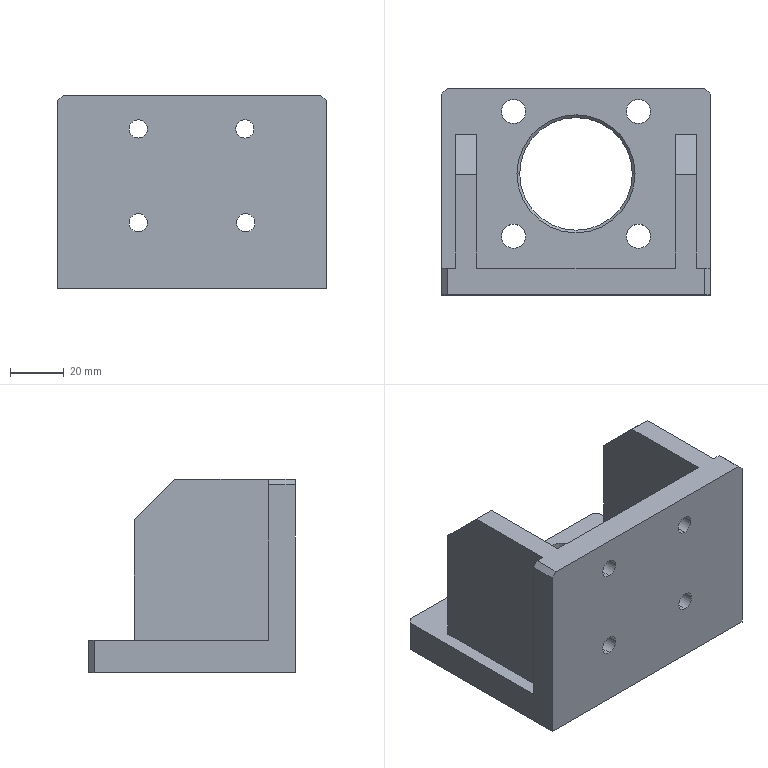Part | STEP file | YCD14007A-08.02.08-Horizontal Cylinder Seat-A3 | 1 solid | 44 faces | box 100 x 77 x 72 mm | volume 177246 mm3 | plane 22 | cylinder 18 | cone 4 | commonest cylinder face diameters 6.8 x8 9 x8 42 x2